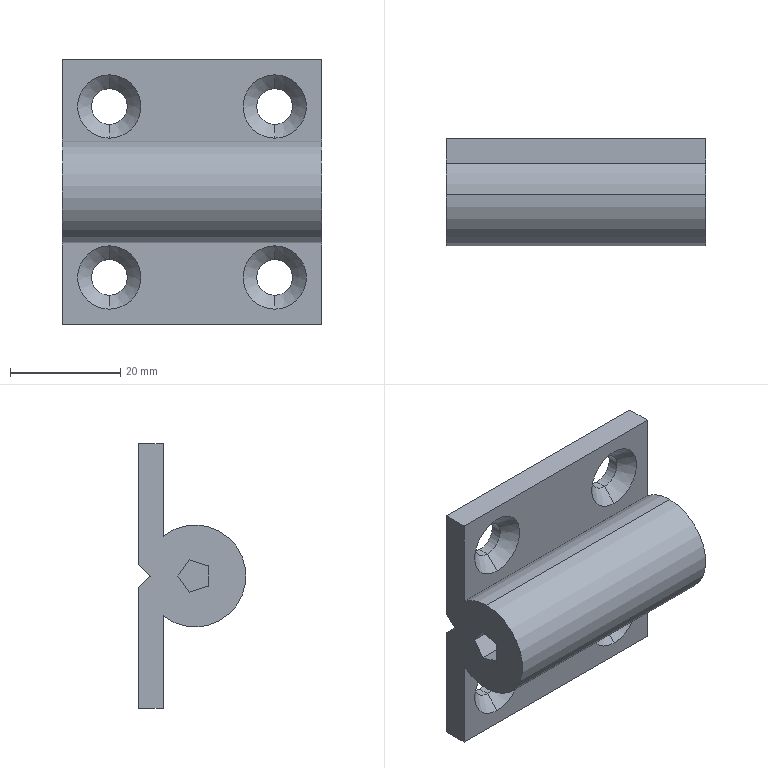Part | STEP file | Damping hinge | 1 solid | 35 faces | box 47 x 19.5 x 48 mm | volume 19859 mm3 | plane 16 | cylinder 11 | cone 8 | commonest cylinder face diameters 6.5 x8 18.5 x3